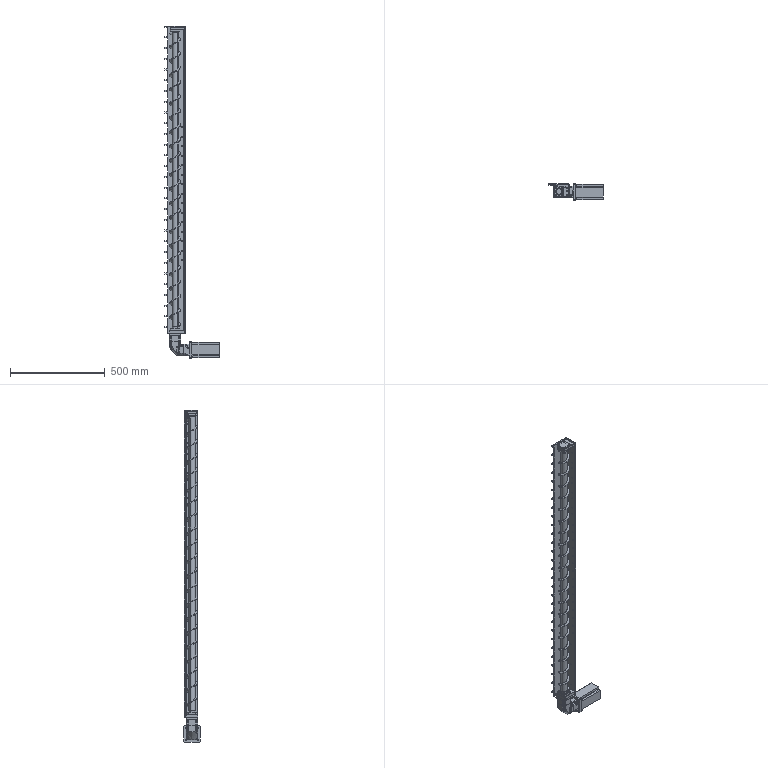Part | SolidWorks | features InContextFeatHolder 8 | 26 solids | 1298 faces | box 286 x 85 x 1747 mm | volume 3499831 mm3 | cylinder 622 | plane 461 | cone 126 | spline 53 | torus 36 | commonest cylinder face diameters 6.8 x120 5.8 x83 4.2 x60 10 x27 69 x26 5.5 x22